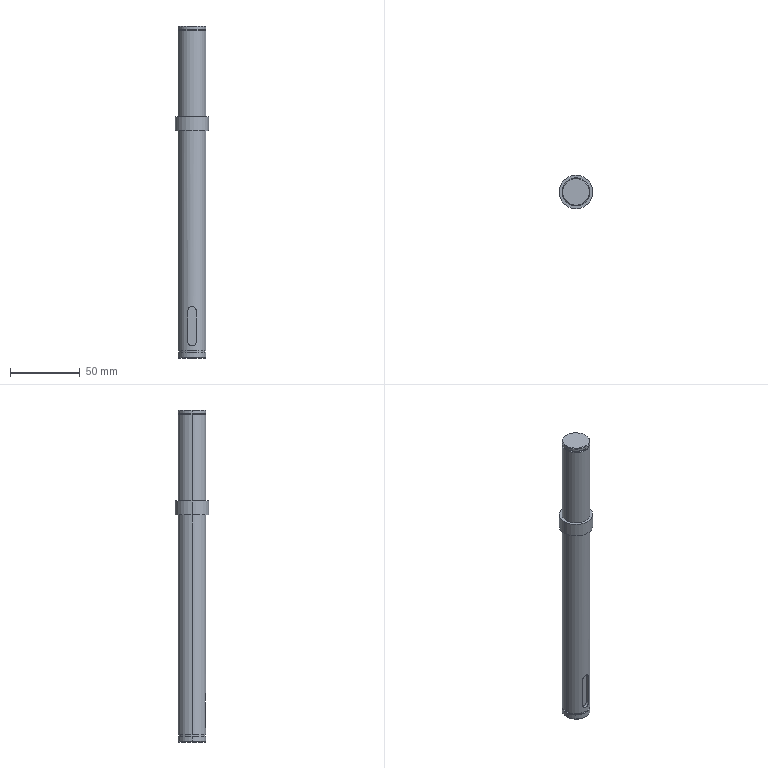Part | SolidWorks | features BaseBody 1 | 1 solid | 31 faces | box 24 x 24 x 237.2 mm | volume 75389 mm3 | cylinder 16 | plane 11 | cone 4 | commonest cylinder face diameters 20 x8 18.35 x4 6 x2 24 x2
STEP:
#1=CARTESIAN_POINT('',(-9.175,0.,233.7));
#2=VERTEX_POINT('',#1);
#3=CARTESIAN_POINT('',(9.175,0.,233.7));
#4=VERTEX_POINT('',#3);
#5=CARTESIAN_POINT('',(0.,0.,233.7));
#6=DIRECTION('',(0.,0.,-1.));
#7=DIRECTION('',(1.,0.,0.));
#8=AXIS2_PLACEMENT_3D('',#5,#6,#7);
#9=CIRCLE('',#8,9.175);
#10=EDGE_CURVE('',#2,#4,#9,.T.);
#11=ORIENTED_EDGE('',*,*,#10,.F.);
#12=CARTESIAN_POINT('',(-9.175,0.,234.9));
#13=VERTEX_POINT('',#12);
#14=CARTESIAN_POINT('',(-9.175,0.,234.3));
#15=DIRECTION('',(0.,0.,1.));
#16=VECTOR('',#15,1000.);
#17=LINE('',#14,#16);
#18=EDGE_CURVE('',#2,#13,#17,.T.);
#19=ORIENTED_EDGE('',*,*,#18,.T.);
#20=CARTESIAN_POINT('',(9.175,0.,234.9));
#21=VERTEX_POINT('',#20);
#22=CARTESIAN_POINT('',(0.,0.,234.9));
#23=DIRECTION('',(0.,0.,-1.));
#24=DIRECTION('',(1.,0.,0.));
#25=AXIS2_PLACEMENT_3D('',#22,#23,#24);
#26=CIRCLE('',#25,9.175);
#27=EDGE_CURVE('',#13,#21,#26,.T.);
#28=ORIENTED_EDGE('',*,*,#27,.T.);
#29=CARTESIAN_POINT('',(9.175,0.,234.3));
#30=DIRECTION('',(0.,0.,1.));
#31=VECTOR('',#30,1000.);
#32=LINE('',#29,#31);
#33=EDGE_CURVE('',#4,#21,#32,.T.);
#34=ORIENTED_EDGE('',*,*,#33,.F.);
#35=EDGE_LOOP('',(#11,#19,#28,#34));
#36=FACE_OUTER_BOUND('',#35,.T.);
#37=CARTESIAN_POINT('',(0.,0.,234.3));
#38=DIRECTION('',(0.,0.,1.));
#39=DIRECTION('',(1.,0.,0.));
#40=AXIS2_PLACEMENT_3D('',#37,#38,#39);
#41=CYLINDRICAL_SURFACE('',#40,9.175);
#42=ADVANCED_FACE('',(#36),#41,.T.);
#43=CARTESIAN_POINT('',(10.,0.,236.7));
#44=VERTEX_POINT('',#43);
#45=CARTESIAN_POINT('',(-10.,0.,236.7));
#46=VERTEX_POINT('',#45);
#47=CARTESIAN_POINT('',(0.,0.,236.7));
#48=DIRECTION('',(0.,0.,1.));
#49=DIRECTION('',(-1.,0.,0.));
#50=AXIS2_PLACEMENT_3D('',#47,#48,#49);
#51=CIRCLE('',#50,10.);
#52=EDGE_CURVE('',#44,#46,#51,.T.);
#53=ORIENTED_EDGE('',*,*,#52,.F.);
#54=CARTESIAN_POINT('',(10.,0.,234.9));
#55=VERTEX_POINT('',#54);
#56=CARTESIAN_POINT('',(10.,0.,0.));
#57=DIRECTION('',(0.,0.,-1.));
#58=VECTOR('',#57,1000.);
#59=LINE('',#56,#58);
#60=EDGE_CURVE('',#44,#55,#59,.T.);
#61=ORIENTED_EDGE('',*,*,#60,.T.);
#62=CARTESIAN_POINT('',(-10.,0.,234.9));
#63=VERTEX_POINT('',#62);
#64=CARTESIAN_POINT('',(0.,0.,234.9));
#65=DIRECTION('',(0.,0.,1.));
#66=DIRECTION('',(-1.,0.,0.));
#67=AXIS2_PLACEMENT_3D('',#64,#65,#66);
#68=CIRCLE('',#67,10.);
#69=EDGE_CURVE('',#55,#63,#68,.T.);
#70=ORIENTED_EDGE('',*,*,#69,.T.);
#71=CARTESIAN_POINT('',(-10.,0.,0.));
#72=DIRECTION('',(0.,0.,-1.));
#73=VECTOR('',#72,1000.);
#74=LINE('',#71,#73);
#75=EDGE_CURVE('',#46,#63,#74,.T.);
#76=ORIENTED_EDGE('',*,*,#75,.F.);
#77=EDGE_LOOP('',(#53,#61,#70,#76));
#78=FACE_OUTER_BOUND('',#77,.T.);
#79=CARTESIAN_POINT('',(0.,0.,0.));
#80=DIRECTION('',(0.,0.,-1.));
#81=DIRECTION('',(-1.,0.,0.));
#82=AXIS2_PLACEMENT_3D('',#79,#80,#81);
#83=CYLINDRICAL_SURFACE('',#82,10.);
#84=ADVANCED_FACE('',(#78),#83,.T.);
#85=CARTESIAN_POINT('',(-9.5,0.,237.2));
#86=VERTEX_POINT('',#85);
#87=CARTESIAN_POINT('',(9.5,0.,237.2));
#88=VERTEX_POINT('',#87);
#89=CARTESIAN_POINT('',(0.,0.,237.2));
#90=DIRECTION('',(0.,0.,-1.));
#91=DIRECTION('',(-1.,0.,0.));
#92=AXIS2_PLACEMENT_3D('',#89,#90,#91);
#93=CIRCLE('',#92,9.5);
#94=EDGE_CURVE('',#86,#88,#93,.T.);
#95=ORIENTED_EDGE('',*,*,#94,.T.);
#96=CARTESIAN_POINT('',(9.75,0.,236.95));
#97=DIRECTION('',(0.7071,0.,-0.7071));
#98=VECTOR('',#97,1000.);
#99=LINE('',#96,#98);
#100=EDGE_CURVE('',#88,#44,#99,.T.);
#101=ORIENTED_EDGE('',*,*,#100,.T.);
#102=ORIENTED_EDGE('',*,*,#52,.T.);
#103=CARTESIAN_POINT('',(-9.75,0.,236.95));
#104=DIRECTION('',(-0.7071,0.,-0.7071));
#105=VECTOR('',#104,1000.);
#106=LINE('',#103,#105);
#107=EDGE_CURVE('',#86,#46,#106,.T.);
#108=ORIENTED_EDGE('',*,*,#107,.F.);
#109=EDGE_LOOP('',(#95,#101,#102,#108));
#110=FACE_OUTER_BOUND('',#109,.T.);
#111=CARTESIAN_POINT('',(0.,0.,236.95));
#112=DIRECTION('',(0.,0.,-1.));
#113=DIRECTION('',(-1.,0.,0.));
#114=AXIS2_PLACEMENT_3D('',#111,#112,#113);
#115=CONICAL_SURFACE('',#114,9.75,0.7854);
#116=ADVANCED_FACE('',(#110),#115,.T.);
#117=CARTESIAN_POINT('',(-10.,0.,233.7));
#118=VERTEX_POINT('',#117);
#119=CARTESIAN_POINT('',(10.,0.,233.7));
#120=VERTEX_POINT('',#119);
#121=CARTESIAN_POINT('',(0.,0.,233.7));
#122=DIRECTION('',(0.,0.,-1.));
#123=DIRECTION('',(-1.,0.,0.));
#124=AXIS2_PLACEMENT_3D('',#121,#122,#123);
#125=CIRCLE('',#124,10.);
#126=EDGE_CURVE('',#118,#120,#125,.T.);
#127=ORIENTED_EDGE('',*,*,#126,.T.);
#128=CARTESIAN_POINT('',(10.,0.,172.2));
#129=VERTEX_POINT('',#128);
#130=CARTESIAN_POINT('',(10.,0.,0.));
#131=DIRECTION('',(0.,0.,-1.));
#132=VECTOR('',#131,1000.);
#133=LINE('',#130,#132);
#134=EDGE_CURVE('',#120,#129,#133,.T.);
#135=ORIENTED_EDGE('',*,*,#134,.T.);
#136=CARTESIAN_POINT('',(-10.,0.,172.2));
#137=VERTEX_POINT('',#136);
#138=CARTESIAN_POINT('',(0.,0.,172.2));
#139=DIRECTION('',(0.,0.,1.));
#140=DIRECTION('',(-1.,0.,0.));
#141=AXIS2_PLACEMENT_3D('',#138,#139,#140);
#142=CIRCLE('',#141,10.);
#143=EDGE_CURVE('',#129,#137,#142,.T.);
#144=ORIENTED_EDGE('',*,*,#143,.T.);
#145=CARTESIAN_POINT('',(-10.,0.,0.));
#146=DIRECTION('',(0.,0.,-1.));
#147=VECTOR('',#146,1000.);
#148=LINE('',#145,#147);
#149=EDGE_CURVE('',#118,#137,#148,.T.);
#150=ORIENTED_EDGE('',*,*,#149,.F.);
#151=EDGE_LOOP('',(#127,#135,#144,#150));
#152=FACE_OUTER_BOUND('',#151,.T.);
#153=CARTESIAN_POINT('',(0.,0.,0.));
#154=DIRECTION('',(0.,0.,-1.));
#155=DIRECTION('',(-1.,0.,0.));
#156=AXIS2_PLACEMENT_3D('',#153,#154,#155);
#157=CYLINDRICAL_SURFACE('',#156,10.);
#158=ADVANCED_FACE('',(#152),#157,.T.);
#159=CARTESIAN_POINT('',(-12.,0.,172.2));
#160=VERTEX_POINT('',#159);
#161=CARTESIAN_POINT('',(12.,0.,172.2));
#162=VERTEX_POINT('',#161);
#163=CARTESIAN_POINT('',(0.,0.,172.2));
#164=DIRECTION('',(0.,0.,1.));
#165=DIRECTION('',(1.,0.,0.));
#166=AXIS2_PLACEMENT_3D('',#163,#164,#165);
#167=CIRCLE('',#166,12.);
#168=EDGE_CURVE('',#160,#162,#167,.T.);
#169=ORIENTED_EDGE('',*,*,#168,.F.);
#170=CARTESIAN_POINT('',(-12.,0.,162.2));
#171=VERTEX_POINT('',#170);
#172=CARTESIAN_POINT('',(-12.,0.,162.2));
#173=DIRECTION('',(0.,0.,-1.));
#174=VECTOR('',#173,1000.);
#175=LINE('',#172,#174);
#176=EDGE_CURVE('',#160,#171,#175,.T.);
#177=ORIENTED_EDGE('',*,*,#176,.T.);
#178=CARTESIAN_POINT('',(12.,0.,162.2));
#179=VERTEX_POINT('',#178);
#180=CARTESIAN_POINT('',(0.,0.,162.2));
#181=DIRECTION('',(0.,0.,1.));
#182=DIRECTION('',(1.,0.,0.));
#183=AXIS2_PLACEMENT_3D('',#180,#181,#182);
#184=CIRCLE('',#183,12.);
#185=EDGE_CURVE('',#171,#179,#184,.T.);
#186=ORIENTED_EDGE('',*,*,#185,.T.);
#187=CARTESIAN_POINT('',(12.,0.,162.2));
#188=DIRECTION('',(0.,0.,-1.));
#189=VECTOR('',#188,1000.);
#190=LINE('',#187,#189);
#191=EDGE_CURVE('',#162,#179,#190,.T.);
#192=ORIENTED_EDGE('',*,*,#191,.F.);
#193=EDGE_LOOP('',(#169,#177,#186,#192));
#194=FACE_OUTER_BOUND('',#193,.T.);
#195=CARTESIAN_POINT('',(0.,0.,162.2));
#196=DIRECTION('',(0.,0.,-1.));
#197=DIRECTION('',(1.,0.,0.));
#198=AXIS2_PLACEMENT_3D('',#195,#196,#197);
#199=CYLINDRICAL_SURFACE('',#198,12.);
#200=ADVANCED_FACE('',(#194),#199,.T.);
#201=CARTESIAN_POINT('',(-10.,0.,162.2));
#202=VERTEX_POINT('',#201);
#203=CARTESIAN_POINT('',(10.,0.,162.2));
#204=VERTEX_POINT('',#203);
#205=CARTESIAN_POINT('',(0.,0.,162.2));
#206=DIRECTION('',(0.,0.,-1.));
#207=DIRECTION('',(-1.,0.,0.));
#208=AXIS2_PLACEMENT_3D('',#205,#206,#207);
#209=CIRCLE('',#208,10.);
#210=EDGE_CURVE('',#202,#204,#209,.T.);
#211=ORIENTED_EDGE('',*,*,#210,.T.);
#212=CARTESIAN_POINT('',(10.,0.,5.2));
#213=VERTEX_POINT('',#212);
#214=CARTESIAN_POINT('',(10.,0.,0.));
#215=DIRECTION('',(0.,0.,-1.));
#216=VECTOR('',#215,1000.);
#217=LINE('',#214,#216);
#218=EDGE_CURVE('',#204,#213,#217,.T.);
#219=ORIENTED_EDGE('',*,*,#218,.T.);
#220=CARTESIAN_POINT('',(-10.,0.,5.2));
#221=VERTEX_POINT('',#220);
#222=CARTESIAN_POINT('',(0.,0.,5.2));
#223=DIRECTION('',(0.,0.,1.));
#224=DIRECTION('',(-1.,0.,0.));
#225=AXIS2_PLACEMENT_3D('',#222,#223,#224);
#226=CIRCLE('',#225,10.);
#227=EDGE_CURVE('',#213,#221,#226,.T.);
#228=ORIENTED_EDGE('',*,*,#227,.T.);
#229=CARTESIAN_POINT('',(-10.,0.,0.));
#230=DIRECTION('',(0.,0.,-1.));
#231=VECTOR('',#230,1000.);
#232=LINE('',#229,#231);
#233=EDGE_CURVE('',#202,#221,#232,.T.);
#234=ORIENTED_EDGE('',*,*,#233,.F.);
#235=EDGE_LOOP('',(#211,#219,#228,#234));
#236=FACE_OUTER_BOUND('',#235,.T.);
#237=CARTESIAN_POINT('',(0.,0.,0.));
#238=DIRECTION('',(0.,0.,-1.));
#239=DIRECTION('',(-1.,0.,0.));
#240=AXIS2_PLACEMENT_3D('',#237,#238,#239);
#241=CYLINDRICAL_SURFACE('',#240,10.);
#242=ADVANCED_FACE('',(#236),#241,.T.);
#243=CARTESIAN_POINT('',(-9.5,0.,0.));
#244=VERTEX_POINT('',#243);
#245=CARTESIAN_POINT('',(9.5,0.,0.));
#246=VERTEX_POINT('',#245);
#247=CARTESIAN_POINT('',(0.,0.,0.));
#248=DIRECTION('',(0.,0.,1.));
#249=DIRECTION('',(-1.,0.,0.));
#250=AXIS2_PLACEMENT_3D('',#247,#248,#249);
#251=CIRCLE('',#250,9.5);
#252=EDGE_CURVE('',#244,#246,#251,.T.);
#253=ORIENTED_EDGE('',*,*,#252,.T.);
#254=CARTESIAN_POINT('',(10.,0.,0.5));
#255=VERTEX_POINT('',#254);
#256=CARTESIAN_POINT('',(9.75,0.,0.25));
#257=DIRECTION('',(0.7071,0.,0.7071));
#258=VECTOR('',#257,1000.);
#259=LINE('',#256,#258);
#260=EDGE_CURVE('',#246,#255,#259,.T.);
#261=ORIENTED_EDGE('',*,*,#260,.T.);
#262=CARTESIAN_POINT('',(-10.,0.,0.5));
#263=VERTEX_POINT('',#262);
#264=CARTESIAN_POINT('',(0.,0.,0.5));
#265=DIRECTION('',(0.,0.,-1.));
#266=DIRECTION('',(-1.,0.,0.));
#267=AXIS2_PLACEMENT_3D('',#264,#265,#266);
#268=CIRCLE('',#267,10.);
#269=EDGE_CURVE('',#255,#263,#268,.T.);
#270=ORIENTED_EDGE('',*,*,#269,.T.);
#271=CARTESIAN_POINT('',(-9.75,0.,0.25));
#272=DIRECTION('',(-0.7071,0.,0.7071));
#273=VECTOR('',#272,1000.);
#274=LINE('',#271,#273);
#275=EDGE_CURVE('',#244,#263,#274,.T.);
#276=ORIENTED_EDGE('',*,*,#275,.F.);
#277=EDGE_LOOP('',(#253,#261,#270,#276));
#278=FACE_OUTER_BOUND('',#277,.T.);
#279=CARTESIAN_POINT('',(0.,0.,0.25));
#280=DIRECTION('',(0.,0.,1.));
#281=DIRECTION('',(-1.,0.,0.));
#282=AXIS2_PLACEMENT_3D('',#279,#280,#281);
#283=CONICAL_SURFACE('',#282,9.75,0.7854);
#284=ADVANCED_FACE('',(#278),#283,.T.);
#285=CARTESIAN_POINT('',(-10.,0.,4.));
#286=VERTEX_POINT('',#285);
#287=CARTESIAN_POINT('',(10.,0.,4.));
#288=VERTEX_POINT('',#287);
#289=CARTESIAN_POINT('',(0.,0.,4.));
#290=DIRECTION('',(0.,0.,-1.));
#291=DIRECTION('',(-1.,0.,0.));
#292=AXIS2_PLACEMENT_3D('',#289,#290,#291);
#293=CIRCLE('',#292,10.);
#294=EDGE_CURVE('',#286,#288,#293,.T.);
#295=ORIENTED_EDGE('',*,*,#294,.T.);
#296=CARTESIAN_POINT('',(10.,0.,0.));
#297=DIRECTION('',(0.,0.,-1.));
#298=VECTOR('',#297,1000.);
#299=LINE('',#296,#298);
#300=EDGE_CURVE('',#288,#255,#299,.T.);
#301=ORIENTED_EDGE('',*,*,#300,.T.);
#302=CARTESIAN_POINT('',(0.,0.,0.5));
#303=DIRECTION('',(0.,0.,-1.));
#304=DIRECTION('',(-1.,0.,0.));
#305=AXIS2_PLACEMENT_3D('',#302,#303,#304);
#306=CIRCLE('',#305,10.);
#307=EDGE_CURVE('',#263,#255,#306,.T.);
#308=ORIENTED_EDGE('',*,*,#307,.F.);
#309=CARTESIAN_POINT('',(-10.,0.,0.));
#310=DIRECTION('',(0.,0.,-1.));
#311=VECTOR('',#310,1000.);
#312=LINE('',#309,#311);
#313=EDGE_CURVE('',#286,#263,#312,.T.);
#314=ORIENTED_EDGE('',*,*,#313,.F.);
#315=EDGE_LOOP('',(#295,#301,#308,#314));
#316=FACE_OUTER_BOUND('',#315,.T.);
#317=CARTESIAN_POINT('',(0.,0.,0.));
#318=DIRECTION('',(0.,0.,-1.));
#319=DIRECTION('',(-1.,0.,0.));
#320=AXIS2_PLACEMENT_3D('',#317,#318,#319);
#321=CYLINDRICAL_SURFACE('',#320,10.);
#322=ADVANCED_FACE('',(#316),#321,.T.);
#323=CARTESIAN_POINT('',(-9.175,0.,4.));
#324=VERTEX_POINT('',#323);
#325=CARTESIAN_POINT('',(9.175,0.,4.));
#326=VERTEX_POINT('',#325);
#327=CARTESIAN_POINT('',(0.,0.,4.));
#328=DIRECTION('',(0.,0.,-1.));
#329=DIRECTION('',(1.,0.,0.));
#330=AXIS2_PLACEMENT_3D('',#327,#328,#329);
#331=CIRCLE('',#330,9.175);
#332=EDGE_CURVE('',#324,#326,#331,.T.);
#333=ORIENTED_EDGE('',*,*,#332,.F.);
#334=CARTESIAN_POINT('',(-9.175,0.,5.2));
#335=VERTEX_POINT('',#334);
#336=CARTESIAN_POINT('',(-9.175,0.,4.6));
#337=DIRECTION('',(0.,0.,1.));
#338=VECTOR('',#337,1000.);
#339=LINE('',#336,#338);
#340=EDGE_CURVE('',#324,#335,#339,.T.);
#341=ORIENTED_EDGE('',*,*,#340,.T.);
#342=CARTESIAN_POINT('',(9.175,0.,5.2));
#343=VERTEX_POINT('',#342);
#344=CARTESIAN_POINT('',(0.,0.,5.2));
#345=DIRECTION('',(0.,0.,-1.));
#346=DIRECTION('',(1.,0.,0.));
#347=AXIS2_PLACEMENT_3D('',#344,#345,#346);
#348=CIRCLE('',#347,9.175);
#349=EDGE_CURVE('',#335,#343,#348,.T.);
#350=ORIENTED_EDGE('',*,*,#349,.T.);
#351=CARTESIAN_POINT('',(9.175,0.,4.6));
#352=DIRECTION('',(0.,0.,1.));
#353=VECTOR('',#352,1000.);
#354=LINE('',#351,#353);
#355=EDGE_CURVE('',#326,#343,#354,.T.);
#356=ORIENTED_EDGE('',*,*,#355,.F.);
#357=EDGE_LOOP('',(#333,#341,#350,#356));
#358=FACE_OUTER_BOUND('',#357,.T.);
#359=CARTESIAN_POINT('',(0.,0.,4.6));
#360=DIRECTION('',(0.,0.,1.));
#361=DIRECTION('',(1.,0.,0.));
#362=AXIS2_PLACEMENT_3D('',#359,#360,#361);
#363=CYLINDRICAL_SURFACE('',#362,9.175);
#364=ADVANCED_FACE('',(#358),#363,.T.);
#365=CARTESIAN_POINT('',(0.,0.,233.7));
#366=DIRECTION('',(0.,0.,-1.));
#367=DIRECTION('',(1.,0.,0.));
#368=AXIS2_PLACEMENT_3D('',#365,#366,#367);
#369=CIRCLE('',#368,9.175);
#370=EDGE_CURVE('',#4,#2,#369,.T.);
#371=ORIENTED_EDGE('',*,*,#370,.T.);
#372=ORIENTED_EDGE('',*,*,#10,.T.);
#373=EDGE_LOOP('',(#371,#372));
#374=FACE_BOUND('',#373,.T.);
#375=ORIENTED_EDGE('',*,*,#126,.F.);
#376=CARTESIAN_POINT('',(0.,0.,233.7));
#377=DIRECTION('',(0.,0.,-1.));
#378=DIRECTION('',(-1.,0.,0.));
#379=AXIS2_PLACEMENT_3D('',#376,#377,#378);
#380=CIRCLE('',#379,10.);
#381=EDGE_CURVE('',#120,#118,#380,.T.);
#382=ORIENTED_EDGE('',*,*,#381,.F.);
#383=EDGE_LOOP('',(#375,#382));
#384=FACE_OUTER_BOUND('',#383,.T.);
#385=CARTESIAN_POINT('',(9.175,0.,233.7));
#386=DIRECTION('',(0.,0.,-1.));
#387=DIRECTION('',(0.,-1.,0.));
#388=AXIS2_PLACEMENT_3D('',#385,#386,#387);
#389=PLANE('',#388);
#390=ADVANCED_FACE('',(#374,#384),#389,.F.);
#391=CARTESIAN_POINT('',(0.,0.,234.9));
#392=DIRECTION('',(0.,0.,-1.));
#393=DIRECTION('',(1.,0.,0.));
#394=AXIS2_PLACEMENT_3D('',#391,#392,#393);
#395=CIRCLE('',#394,9.175);
#396=EDGE_CURVE('',#21,#13,#395,.T.);
#397=ORIENTED_EDGE('',*,*,#396,.F.);
#398=ORIENTED_EDGE('',*,*,#27,.F.);
#399=EDGE_LOOP('',(#397,#398));
#400=FACE_BOUND('',#399,.T.);
#401=CARTESIAN_POINT('',(0.,0.,234.9));
#402=DIRECTION('',(0.,0.,1.));
#403=DIRECTION('',(-1.,0.,0.));
#404=AXIS2_PLACEMENT_3D('',#401,#402,#403);
#405=CIRCLE('',#404,10.);
#406=EDGE_CURVE('',#63,#55,#405,.T.);
#407=ORIENTED_EDGE('',*,*,#406,.F.);
#408=ORIENTED_EDGE('',*,*,#69,.F.);
#409=EDGE_LOOP('',(#407,#408));
#410=FACE_OUTER_BOUND('',#409,.T.);
#411=CARTESIAN_POINT('',(12.,0.,234.9));
#412=DIRECTION('',(0.,0.,1.));
#413=DIRECTION('',(1.,0.,0.));
#414=AXIS2_PLACEMENT_3D('',#411,#412,#413);
#415=PLANE('',#414);
#416=ADVANCED_FACE('',(#400,#410),#415,.F.);
#417=ORIENTED_EDGE('',*,*,#94,.F.);
#418=CARTESIAN_POINT('',(0.,0.,237.2));
#419=DIRECTION('',(0.,0.,-1.));
#420=DIRECTION('',(-1.,0.,0.));
#421=AXIS2_PLACEMENT_3D('',#418,#419,#420);
#422=CIRCLE('',#421,9.5);
#423=EDGE_CURVE('',#88,#86,#422,.T.);
#424=ORIENTED_EDGE('',*,*,#423,.F.);
#425=EDGE_LOOP('',(#417,#424));
#426=FACE_OUTER_BOUND('',#425,.T.);
#427=CARTESIAN_POINT('',(0.,0.,237.2));
#428=DIRECTION('',(0.,0.,1.));
#429=DIRECTION('',(1.,0.,0.));
#430=AXIS2_PLACEMENT_3D('',#427,#428,#429);
#431=PLANE('',#430);
#432=ADVANCED_FACE('',(#426),#431,.T.);
#433=CARTESIAN_POINT('',(0.,0.,172.2));
#434=DIRECTION('',(0.,0.,1.));
#435=DIRECTION('',(-1.,0.,0.));
#436=AXIS2_PLACEMENT_3D('',#433,#434,#435);
#437=CIRCLE('',#436,10.);
#438=EDGE_CURVE('',#137,#129,#437,.T.);
#439=ORIENTED_EDGE('',*,*,#438,.F.);
#440=ORIENTED_EDGE('',*,*,#143,.F.);
#441=EDGE_LOOP('',(#439,#440));
#442=FACE_BOUND('',#441,.T.);
#443=CARTESIAN_POINT('',(0.,0.,172.2));
#444=DIRECTION('',(0.,0.,1.));
#445=DIRECTION('',(1.,0.,0.));
#446=AXIS2_PLACEMENT_3D('',#443,#444,#445);
#447=CIRCLE('',#446,12.);
#448=EDGE_CURVE('',#162,#160,#447,.T.);
#449=ORIENTED_EDGE('',*,*,#448,.T.);
#450=ORIENTED_EDGE('',*,*,#168,.T.);
#451=EDGE_LOOP('',(#449,#450));
#452=FACE_OUTER_BOUND('',#451,.T.);
#453=CARTESIAN_POINT('',(0.,0.,172.2));
#454=DIRECTION('',(0.,0.,1.));
#455=DIRECTION('',(1.,0.,0.));
#456=AXIS2_PLACEMENT_3D('',#453,#454,#455);
#457=PLANE('',#456);
#458=ADVANCED_FACE('',(#442,#452),#457,.T.);
#459=ORIENTED_EDGE('',*,*,#210,.F.);
#460=CARTESIAN_POINT('',(0.,0.,162.2));
#461=DIRECTION('',(0.,0.,-1.));
#462=DIRECTION('',(-1.,0.,0.));
#463=AXIS2_PLACEMENT_3D('',#460,#461,#462);
#464=CIRCLE('',#463,10.);
#465=EDGE_CURVE('',#204,#202,#464,.T.);
#466=ORIENTED_EDGE('',*,*,#465,.F.);
#467=EDGE_LOOP('',(#459,#466));
#468=FACE_BOUND('',#467,.T.);
#469=CARTESIAN_POINT('',(0.,0.,162.2));
#470=DIRECTION('',(0.,0.,1.));
#471=DIRECTION('',(1.,0.,0.));
#472=AXIS2_PLACEMENT_3D('',#469,#470,#471);
#473=CIRCLE('',#472,12.);
#474=EDGE_CURVE('',#179,#171,#473,.T.);
#475=ORIENTED_EDGE('',*,*,#474,.F.);
#476=ORIENTED_EDGE('',*,*,#185,.F.);
#477=EDGE_LOOP('',(#475,#476));
#478=FACE_OUTER_BOUND('',#477,.T.);
#479=CARTESIAN_POINT('',(0.,0.,162.2));
#480=DIRECTION('',(0.,0.,1.));
#481=DIRECTION('',(1.,0.,0.));
#482=AXIS2_PLACEMENT_3D('',#479,#480,#481);
#483=PLANE('',#482);
#484=ADVANCED_FACE('',(#468,#478),#483,.F.);
#485=ORIENTED_EDGE('',*,*,#252,.F.);
#486=CARTESIAN_POINT('',(0.,0.,0.));
#487=DIRECTION('',(0.,0.,1.));
#488=DIRECTION('',(-1.,0.,0.));
#489=AXIS2_PLACEMENT_3D('',#486,#487,#488);
#490=CIRCLE('',#489,9.5);
#491=EDGE_CURVE('',#246,#244,#490,.T.);
#492=ORIENTED_EDGE('',*,*,#491,.F.);
#493=EDGE_LOOP('',(#485,#492));
#494=FACE_OUTER_BOUND('',#493,.T.);
#495=CARTESIAN_POINT('',(0.,0.,0.));
#496=DIRECTION('',(0.,0.,1.));
#497=DIRECTION('',(1.,0.,0.));
#498=AXIS2_PLACEMENT_3D('',#495,#496,#497);
#499=PLANE('',#498);
#500=ADVANCED_FACE('',(#494),#499,.F.);
#501=CARTESIAN_POINT('',(0.,0.,4.));
#502=DIRECTION('',(0.,0.,-1.));
#503=DIRECTION('',(1.,0.,0.));
#504=AXIS2_PLACEMENT_3D('',#501,#502,#503);
#505=CIRCLE('',#504,9.175);
#506=EDGE_CURVE('',#326,#324,#505,.T.);
#507=ORIENTED_EDGE('',*,*,#506,.T.);
#508=ORIENTED_EDGE('',*,*,#332,.T.);
#509=EDGE_LOOP('',(#507,#508));
#510=FACE_BOUND('',#509,.T.);
#511=ORIENTED_EDGE('',*,*,#294,.F.);
#512=CARTESIAN_POINT('',(0.,0.,4.));
#513=DIRECTION('',(0.,0.,-1.));
#514=DIRECTION('',(-1.,0.,0.));
#515=AXIS2_PLACEMENT_3D('',#512,#513,#514);
#516=CIRCLE('',#515,10.);
#517=EDGE_CURVE('',#288,#286,#516,.T.);
#518=ORIENTED_EDGE('',*,*,#517,.F.);
#519=EDGE_LOOP('',(#511,#518));
#520=FACE_OUTER_BOUND('',#519,.T.);
#521=CARTESIAN_POINT('',(9.175,0.,4.));
#522=DIRECTION('',(0.,0.,-1.));
#523=DIRECTION('',(0.,-1.,0.));
#524=AXIS2_PLACEMENT_3D('',#521,#522,#523);
#525=PLANE('',#524);
#526=ADVANCED_FACE('',(#510,#520),#525,.F.);
#527=CARTESIAN_POINT('',(0.,0.,5.2));
#528=DIRECTION('',(0.,0.,-1.));
#529=DIRECTION('',(1.,0.,0.));
#530=AXIS2_PLACEMENT_3D('',#527,#528,#529);
#531=CIRCLE('',#530,9.175);
#532=EDGE_CURVE('',#343,#335,#531,.T.);
#533=ORIENTED_EDGE('',*,*,#532,.F.);
#534=ORIENTED_EDGE('',*,*,#349,.F.);
#535=EDGE_LOOP('',(#533,#534));
#536=FACE_BOUND('',#535,.T.);
#537=CARTESIAN_POINT('',(0.,0.,5.2));
#538=DIRECTION('',(0.,0.,1.));
#539=DIRECTION('',(-1.,0.,0.));
#540=AXIS2_PLACEMENT_3D('',#537,#538,#539);
#541=CIRCLE('',#540,10.);
#542=EDGE_CURVE('',#221,#213,#541,.T.);
#543=ORIENTED_EDGE('',*,*,#542,.F.);
#544=ORIENTED_EDGE('',*,*,#227,.F.);
#545=EDGE_LOOP('',(#543,#544));
#546=FACE_OUTER_BOUND('',#545,.T.);
#547=CARTESIAN_POINT('',(16.183,0.,5.2));
#548=DIRECTION('',(0.,0.,1.));
#549=DIRECTION('',(1.,0.,0.));
#550=AXIS2_PLACEMENT_3D('',#547,#548,#549);
#551=PLANE('',#550);
#552=ADVANCED_FACE('',(#536,#546),#551,.F.);
#553=CARTESIAN_POINT('',(-3.,-9.539,11.7));
#554=VERTEX_POINT('',#553);
#555=CARTESIAN_POINT('',(-3.,-9.539,33.7));
#556=VERTEX_POINT('',#555);
#557=CARTESIAN_POINT('',(-3.,-9.539,0.));
#558=DIRECTION('',(0.,0.,1.));
#559=VECTOR('',#558,1000.);
#560=LINE('',#557,#559);
#561=EDGE_CURVE('',#554,#556,#560,.T.);
#562=ORIENTED_EDGE('',*,*,#561,.F.);
#563=CARTESIAN_POINT('',(-3.,-7.5,11.7));
#564=VERTEX_POINT('',#563);
#565=CARTESIAN_POINT('',(-3.,-10.,11.7));
#566=DIRECTION('',(0.,1.,0.));
#567=VECTOR('',#566,1000.);
#568=LINE('',#565,#567);
#569=EDGE_CURVE('',#554,#564,#568,.T.);
#570=ORIENTED_EDGE('',*,*,#569,.T.);
#571=CARTESIAN_POINT('',(-3.,-7.5,33.7));
#572=VERTEX_POINT('',#571);
#573=CARTESIAN_POINT('',(-3.,-7.5,11.7));
#574=DIRECTION('',(0.,0.,1.));
#575=VECTOR('',#574,1000.);
#576=LINE('',#573,#575);
#577=EDGE_CURVE('',#564,#572,#576,.T.);
#578=ORIENTED_EDGE('',*,*,#577,.T.);
#579=CARTESIAN_POINT('',(-3.,-10.,33.7));
#580=DIRECTION('',(0.,1.,0.));
#581=VECTOR('',#580,1000.);
#582=LINE('',#579,#581);
#583=EDGE_CURVE('',#556,#572,#582,.T.);
#584=ORIENTED_EDGE('',*,*,#583,.F.);
#585=EDGE_LOOP('',(#562,#570,#578,#584));
#586=FACE_OUTER_BOUND('',#585,.T.);
#587=CARTESIAN_POINT('',(-3.,-10.,11.7));
#588=DIRECTION('',(-1.,0.,0.));
#589=DIRECTION('',(0.,0.,1.));
#590=AXIS2_PLACEMENT_3D('',#587,#588,#589);
#591=PLANE('',#590);
#592=ADVANCED_FACE('',(#586),#591,.F.);
#593=CARTESIAN_POINT('',(3.,-9.539,33.7));
#594=VERTEX_POINT('',#593);
#595=CARTESIAN_POINT('',(-3.,-9.539,33.7));
#596=CARTESIAN_POINT('',(-3.,-9.539,33.899));
#597=CARTESIAN_POINT('',(-2.98,-9.546,34.095));
#598=CARTESIAN_POINT('',(-2.904,-9.569,34.48));
#599=CARTESIAN_POINT('',(-2.845,-9.587,34.671));
#600=CARTESIAN_POINT('',(-2.695,-9.63,35.033));
#601=CARTESIAN_POINT('',(-2.602,-9.656,35.205));
#602=CARTESIAN_POINT('',(-2.385,-9.712,35.53));
#603=CARTESIAN_POINT('',(-2.259,-9.742,35.683));
#604=CARTESIAN_POINT('',(-1.847,-9.832,36.096));
#605=CARTESIAN_POINT('',(-1.515,-9.891,36.319));
#606=CARTESIAN_POINT('',(-0.9743,-9.954,36.544));
#607=CARTESIAN_POINT('',(-0.7844,-9.971,36.602));
#608=CARTESIAN_POINT('',(-0.396,-9.994,36.68));
#609=CARTESIAN_POINT('',(-0.1993,-10.,36.7));
#610=CARTESIAN_POINT('',(0.1994,-10.,36.7));
#611=CARTESIAN_POINT('',(0.3951,-9.994,36.68));
#612=CARTESIAN_POINT('',(0.7799,-9.971,36.603));
#613=CARTESIAN_POINT('',(0.971,-9.954,36.545));
#614=CARTESIAN_POINT('',(1.334,-9.912,36.394));
#615=CARTESIAN_POINT('',(1.505,-9.887,36.302));
#616=CARTESIAN_POINT('',(1.831,-9.832,36.085));
#617=CARTESIAN_POINT('',(1.984,-9.802,35.959));
#618=CARTESIAN_POINT('',(2.396,-9.713,35.547));
#619=CARTESIAN_POINT('',(2.619,-9.652,35.214));
#620=CARTESIAN_POINT('',(2.844,-9.587,34.674));
#621=CARTESIAN_POINT('',(2.902,-9.57,34.484));
#622=CARTESIAN_POINT('',(2.98,-9.546,34.096));
#623=CARTESIAN_POINT('',(3.,-9.539,33.899));
#624=CARTESIAN_POINT('',(3.,-9.539,33.7));
#625=B_SPLINE_CURVE_WITH_KNOTS('',3,(#595,#596,#597,#598,#599,#600,#601,#602,#603,#604,#605,#606,#607,#608,#609,#610,#611,#612,#613,#614,#615,#616,#617,#618,#619,#620,#621,#622,#623,#624),.UNSPECIFIED.,.F.,.F.,(4,2,2,2,2,2,2,2,2,2,2,2,2,2,4),(0.,0.0005892,0.001178,0.001768,0.002357,0.003535,0.004125,0.004714,0.005303,0.005892,0.006482,0.007071,0.008249,0.008838,0.009428),.UNSPECIFIED.);
#626=EDGE_CURVE('',#556,#594,#625,.T.);
#627=ORIENTED_EDGE('',*,*,#626,.F.);
#628=ORIENTED_EDGE('',*,*,#583,.T.);
#629=CARTESIAN_POINT('',(3.,-7.5,33.7));
#630=VERTEX_POINT('',#629);
#631=CARTESIAN_POINT('',(0.,-7.5,33.7));
#632=DIRECTION('',(0.,1.,0.));
#633=DIRECTION('',(-1.,0.,0.));
#634=AXIS2_PLACEMENT_3D('',#631,#632,#633);
#635=CIRCLE('',#634,3.);
#636=EDGE_CURVE('',#572,#630,#635,.T.);
#637=ORIENTED_EDGE('',*,*,#636,.T.);
#638=CARTESIAN_POINT('',(3.,-10.,33.7));
#639=DIRECTION('',(0.,1.,0.));
#640=VECTOR('',#639,1000.);
#641=LINE('',#638,#640);
#642=EDGE_CURVE('',#594,#630,#641,.T.);
#643=ORIENTED_EDGE('',*,*,#642,.F.);
#644=EDGE_LOOP('',(#627,#628,#637,#643));
#645=FACE_OUTER_BOUND('',#644,.T.);
#646=CARTESIAN_POINT('',(0.,-10.,33.7));
#647=DIRECTION('',(0.,-1.,0.));
#648=DIRECTION('',(-1.,0.,0.));
#649=AXIS2_PLACEMENT_3D('',#646,#647,#648);
#650=CYLINDRICAL_SURFACE('',#649,3.);
#651=ADVANCED_FACE('',(#645),#650,.F.);
#652=CARTESIAN_POINT('',(3.,-9.539,11.7));
#653=VERTEX_POINT('',#652);
#654=CARTESIAN_POINT('',(3.,-9.539,0.));
#655=DIRECTION('',(0.,0.,-1.));
#656=VECTOR('',#655,1000.);
#657=LINE('',#654,#656);
#658=EDGE_CURVE('',#594,#653,#657,.T.);
#659=ORIENTED_EDGE('',*,*,#658,.F.);
#660=ORIENTED_EDGE('',*,*,#642,.T.);
#661=CARTESIAN_POINT('',(3.,-7.5,11.7));
#662=VERTEX_POINT('',#661);
#663=CARTESIAN_POINT('',(3.,-7.5,33.7));
#664=DIRECTION('',(0.,0.,-1.));
#665=VECTOR('',#664,1000.);
#666=LINE('',#663,#665);
#667=EDGE_CURVE('',#630,#662,#666,.T.);
#668=ORIENTED_EDGE('',*,*,#667,.T.);
#669=CARTESIAN_POINT('',(3.,-10.,11.7));
#670=DIRECTION('',(0.,1.,0.));
#671=VECTOR('',#670,1000.);
#672=LINE('',#669,#671);
#673=EDGE_CURVE('',#653,#662,#672,.T.);
#674=ORIENTED_EDGE('',*,*,#673,.F.);
#675=EDGE_LOOP('',(#659,#660,#668,#674));
#676=FACE_OUTER_BOUND('',#675,.T.);
#677=CARTESIAN_POINT('',(3.,-10.,33.7));
#678=DIRECTION('',(1.,0.,0.));
#679=DIRECTION('',(0.,1.,0.));
#680=AXIS2_PLACEMENT_3D('',#677,#678,#679);
#681=PLANE('',#680);
#682=ADVANCED_FACE('',(#676),#681,.F.);
#683=CARTESIAN_POINT('',(3.,-9.539,11.7));
#684=CARTESIAN_POINT('',(3.,-9.539,11.501));
#685=CARTESIAN_POINT('',(2.98,-9.546,11.305));
#686=CARTESIAN_POINT('',(2.904,-9.569,10.92));
#687=CARTESIAN_POINT('',(2.845,-9.587,10.729));
#688=CARTESIAN_POINT('',(2.695,-9.63,10.367));
#689=CARTESIAN_POINT('',(2.602,-9.656,10.195));
#690=CARTESIAN_POINT('',(2.385,-9.712,9.87));
#691=CARTESIAN_POINT('',(2.259,-9.742,9.717));
#692=CARTESIAN_POINT('',(1.847,-9.832,9.304));
#693=CARTESIAN_POINT('',(1.515,-9.891,9.081));
#694=CARTESIAN_POINT('',(0.9743,-9.954,8.856));
#695=CARTESIAN_POINT('',(0.7844,-9.971,8.798));
#696=CARTESIAN_POINT('',(0.396,-9.994,8.72));
#697=CARTESIAN_POINT('',(0.1993,-10.,8.7));
#698=CARTESIAN_POINT('',(-0.1994,-10.,8.7));
#699=CARTESIAN_POINT('',(-0.3951,-9.994,8.72));
#700=CARTESIAN_POINT('',(-0.7799,-9.971,8.797));
#701=CARTESIAN_POINT('',(-0.971,-9.954,8.855));
#702=CARTESIAN_POINT('',(-1.334,-9.912,9.006));
#703=CARTESIAN_POINT('',(-1.505,-9.887,9.098));
#704=CARTESIAN_POINT('',(-1.831,-9.832,9.315));
#705=CARTESIAN_POINT('',(-1.984,-9.802,9.441));
#706=CARTESIAN_POINT('',(-2.396,-9.713,9.853));
#707=CARTESIAN_POINT('',(-2.619,-9.652,10.186));
#708=CARTESIAN_POINT('',(-2.844,-9.587,10.726));
#709=CARTESIAN_POINT('',(-2.902,-9.57,10.916));
#710=CARTESIAN_POINT('',(-2.98,-9.546,11.304));
#711=CARTESIAN_POINT('',(-3.,-9.539,11.501));
#712=CARTESIAN_POINT('',(-3.,-9.539,11.7));
#713=B_SPLINE_CURVE_WITH_KNOTS('',3,(#683,#684,#685,#686,#687,#688,#689,#690,#691,#692,#693,#694,#695,#696,#697,#698,#699,#700,#701,#702,#703,#704,#705,#706,#707,#708,#709,#710,#711,#712),.UNSPECIFIED.,.F.,.F.,(4,2,2,2,2,2,2,2,2,2,2,2,2,2,4),(-0.004714,-0.004125,-0.003535,-0.002946,-0.002357,-0.001178,-0.0005892,0.000000044,0.0005893,0.001179,0.001768,0.002357,0.003535,0.004125,0.004714),.UNSPECIFIED.);
#714=EDGE_CURVE('',#653,#554,#713,.T.);
#715=ORIENTED_EDGE('',*,*,#714,.F.);
#716=ORIENTED_EDGE('',*,*,#673,.T.);
#717=CARTESIAN_POINT('',(0.,-7.5,11.7));
#718=DIRECTION('',(0.,1.,0.));
#719=DIRECTION('',(1.,0.,0.));
#720=AXIS2_PLACEMENT_3D('',#717,#718,#719);
#721=CIRCLE('',#720,3.);
#722=EDGE_CURVE('',#662,#564,#721,.T.);
#723=ORIENTED_EDGE('',*,*,#722,.T.);
#724=ORIENTED_EDGE('',*,*,#569,.F.);
#725=EDGE_LOOP('',(#715,#716,#723,#724));
#726=FACE_OUTER_BOUND('',#725,.T.);
#727=CARTESIAN_POINT('',(0.,-10.,11.7));
#728=DIRECTION('',(0.,-1.,0.));
#729=DIRECTION('',(1.,0.,0.));
#730=AXIS2_PLACEMENT_3D('',#727,#728,#729);
#731=CYLINDRICAL_SURFACE('',#730,3.);
#732=ADVANCED_FACE('',(#726),#731,.F.);
#733=ORIENTED_EDGE('',*,*,#636,.F.);
#734=ORIENTED_EDGE('',*,*,#577,.F.);
#735=ORIENTED_EDGE('',*,*,#722,.F.);
#736=ORIENTED_EDGE('',*,*,#667,.F.);
#737=EDGE_LOOP('',(#733,#734,#735,#736));
#738=FACE_OUTER_BOUND('',#737,.T.);
#739=CARTESIAN_POINT('',(0.,-7.5,34.733));
#740=DIRECTION('',(0.,1.,0.));
#741=DIRECTION('',(1.,0.,0.));
#742=AXIS2_PLACEMENT_3D('',#739,#740,#741);
#743=PLANE('',#742);
#744=ADVANCED_FACE('',(#738),#743,.F.);
#745=ORIENTED_EDGE('',*,*,#340,.F.);
#746=ORIENTED_EDGE('',*,*,#506,.F.);
#747=ORIENTED_EDGE('',*,*,#355,.T.);
#748=ORIENTED_EDGE('',*,*,#532,.T.);
#749=EDGE_LOOP('',(#745,#746,#747,#748));
#750=FACE_OUTER_BOUND('',#749,.T.);
#751=CARTESIAN_POINT('',(0.,0.,4.6));
#752=DIRECTION('',(0.,0.,1.));
#753=DIRECTION('',(1.,0.,0.));
#754=AXIS2_PLACEMENT_3D('',#751,#752,#753);
#755=CYLINDRICAL_SURFACE('',#754,9.175);
#756=ADVANCED_FACE('',(#750),#755,.T.);
#757=ORIENTED_EDGE('',*,*,#300,.F.);
#758=ORIENTED_EDGE('',*,*,#517,.T.);
#759=ORIENTED_EDGE('',*,*,#313,.T.);
#760=ORIENTED_EDGE('',*,*,#269,.F.);
#761=EDGE_LOOP('',(#757,#758,#759,#760));
#762=FACE_OUTER_BOUND('',#761,.T.);
#763=CARTESIAN_POINT('',(0.,0.,0.));
#764=DIRECTION('',(0.,0.,-1.));
#765=DIRECTION('',(-1.,0.,0.));
#766=AXIS2_PLACEMENT_3D('',#763,#764,#765);
#767=CYLINDRICAL_SURFACE('',#766,10.);
#768=ADVANCED_FACE('',(#762),#767,.T.);
#769=ORIENTED_EDGE('',*,*,#260,.F.);
#770=ORIENTED_EDGE('',*,*,#491,.T.);
#771=ORIENTED_EDGE('',*,*,#275,.T.);
#772=ORIENTED_EDGE('',*,*,#307,.T.);
#773=EDGE_LOOP('',(#769,#770,#771,#772));
#774=FACE_OUTER_BOUND('',#773,.T.);
#775=CARTESIAN_POINT('',(0.,0.,0.25));
#776=DIRECTION('',(0.,0.,1.));
#777=DIRECTION('',(-1.,0.,0.));
#778=AXIS2_PLACEMENT_3D('',#775,#776,#777);
#779=CONICAL_SURFACE('',#778,9.75,0.7854);
#780=ADVANCED_FACE('',(#774),#779,.T.);
#781=ORIENTED_EDGE('',*,*,#218,.F.);
#782=ORIENTED_EDGE('',*,*,#465,.T.);
#783=ORIENTED_EDGE('',*,*,#233,.T.);
#784=ORIENTED_EDGE('',*,*,#542,.T.);
#785=EDGE_LOOP('',(#781,#782,#783,#784));
#786=FACE_OUTER_BOUND('',#785,.T.);
#787=ORIENTED_EDGE('',*,*,#658,.T.);
#788=ORIENTED_EDGE('',*,*,#714,.T.);
#789=ORIENTED_EDGE('',*,*,#561,.T.);
#790=ORIENTED_EDGE('',*,*,#626,.T.);
#791=EDGE_LOOP('',(#787,#788,#789,#790));
#792=FACE_BOUND('',#791,.T.);
#793=CARTESIAN_POINT('',(0.,0.,0.));
#794=DIRECTION('',(0.,0.,-1.));
#795=DIRECTION('',(-1.,0.,0.));
#796=AXIS2_PLACEMENT_3D('',#793,#794,#795);
#797=CYLINDRICAL_SURFACE('',#796,10.);
#798=ADVANCED_FACE('',(#786,#792),#797,.T.);
#799=ORIENTED_EDGE('',*,*,#176,.F.);
#800=ORIENTED_EDGE('',*,*,#448,.F.);
#801=ORIENTED_EDGE('',*,*,#191,.T.);
#802=ORIENTED_EDGE('',*,*,#474,.T.);
#803=EDGE_LOOP('',(#799,#800,#801,#802));
#804=FACE_OUTER_BOUND('',#803,.T.);
#805=CARTESIAN_POINT('',(0.,0.,162.2));
#806=DIRECTION('',(0.,0.,-1.));
#807=DIRECTION('',(1.,0.,0.));
#808=AXIS2_PLACEMENT_3D('',#805,#806,#807);
#809=CYLINDRICAL_SURFACE('',#808,12.);
#810=ADVANCED_FACE('',(#804),#809,.T.);
#811=ORIENTED_EDGE('',*,*,#134,.F.);
#812=ORIENTED_EDGE('',*,*,#381,.T.);
#813=ORIENTED_EDGE('',*,*,#149,.T.);
#814=ORIENTED_EDGE('',*,*,#438,.T.);
#815=EDGE_LOOP('',(#811,#812,#813,#814));
#816=FACE_OUTER_BOUND('',#815,.T.);
#817=CARTESIAN_POINT('',(0.,0.,0.));
#818=DIRECTION('',(0.,0.,-1.));
#819=DIRECTION('',(-1.,0.,0.));
#820=AXIS2_PLACEMENT_3D('',#817,#818,#819);
#821=CYLINDRICAL_SURFACE('',#820,10.);
#822=ADVANCED_FACE('',(#816),#821,.T.);
#823=ORIENTED_EDGE('',*,*,#100,.F.);
#824=ORIENTED_EDGE('',*,*,#423,.T.);
#825=ORIENTED_EDGE('',*,*,#107,.T.);
#826=CARTESIAN_POINT('',(0.,0.,236.7));
#827=DIRECTION('',(0.,0.,1.));
#828=DIRECTION('',(-1.,0.,0.));
#829=AXIS2_PLACEMENT_3D('',#826,#827,#828);
#830=CIRCLE('',#829,10.);
#831=EDGE_CURVE('',#46,#44,#830,.T.);
#832=ORIENTED_EDGE('',*,*,#831,.T.);
#833=EDGE_LOOP('',(#823,#824,#825,#832));
#834=FACE_OUTER_BOUND('',#833,.T.);
#835=CARTESIAN_POINT('',(0.,0.,236.95));
#836=DIRECTION('',(0.,0.,-1.));
#837=DIRECTION('',(-1.,0.,0.));
#838=AXIS2_PLACEMENT_3D('',#835,#836,#837);
#839=CONICAL_SURFACE('',#838,9.75,0.7854);
#840=ADVANCED_FACE('',(#834),#839,.T.);
#841=ORIENTED_EDGE('',*,*,#60,.F.);
#842=ORIENTED_EDGE('',*,*,#831,.F.);
#843=ORIENTED_EDGE('',*,*,#75,.T.);
#844=ORIENTED_EDGE('',*,*,#406,.T.);
#845=EDGE_LOOP('',(#841,#842,#843,#844));
#846=FACE_OUTER_BOUND('',#845,.T.);
#847=CARTESIAN_POINT('',(0.,0.,0.));
#848=DIRECTION('',(0.,0.,-1.));
#849=DIRECTION('',(-1.,0.,0.));
#850=AXIS2_PLACEMENT_3D('',#847,#848,#849);
#851=CYLINDRICAL_SURFACE('',#850,10.);
#852=ADVANCED_FACE('',(#846),#851,.T.);
#853=ORIENTED_EDGE('',*,*,#18,.F.);
#854=ORIENTED_EDGE('',*,*,#370,.F.);
#855=ORIENTED_EDGE('',*,*,#33,.T.);
#856=ORIENTED_EDGE('',*,*,#396,.T.);
#857=EDGE_LOOP('',(#853,#854,#855,#856));
#858=FACE_OUTER_BOUND('',#857,.T.);
#859=CARTESIAN_POINT('',(0.,0.,234.3));
#860=DIRECTION('',(0.,0.,1.));
#861=DIRECTION('',(1.,0.,0.));
#862=AXIS2_PLACEMENT_3D('',#859,#860,#861);
#863=CYLINDRICAL_SURFACE('',#862,9.175);
#864=ADVANCED_FACE('',(#858),#863,.T.);
#865=CLOSED_SHELL('',(#42,#84,#116,#158,#200,#242,#284,#322,#364,#390,#416,#432,#458,#484,#500,#526,#552,#592,#651,#682,#732,#744,#756,#768,#780,#798,#810,#822,#840,#852,#864));
#866=MANIFOLD_SOLID_BREP('',#865);
#867=CARTESIAN_POINT('',(0.,0.,0.));
#868=DIRECTION('',(0.,0.,1.));
#869=DIRECTION('',(1.,0.,0.));
#870=AXIS2_PLACEMENT_3D('',#867,#868,#869);
#871=(LENGTH_UNIT()NAMED_UNIT(*)SI_UNIT(.MILLI.,.METRE.));
#872=UNCERTAINTY_MEASURE_WITH_UNIT(LENGTH_MEASURE(0.00001),#871,'','');
#873=(NAMED_UNIT(*)PLANE_ANGLE_UNIT()SI_UNIT($,.RADIAN.));
#874=(NAMED_UNIT(*)SI_UNIT($,.STERADIAN.)SOLID_ANGLE_UNIT());
#875=(GEOMETRIC_REPRESENTATION_CONTEXT(3)GLOBAL_UNCERTAINTY_ASSIGNED_CONTEXT((#872))GLOBAL_UNIT_ASSIGNED_CONTEXT((#871,#873,#874))REPRESENTATION_CONTEXT('',''));
#876=ADVANCED_BREP_SHAPE_REPRESENTATION('',(#866,#870),#875);